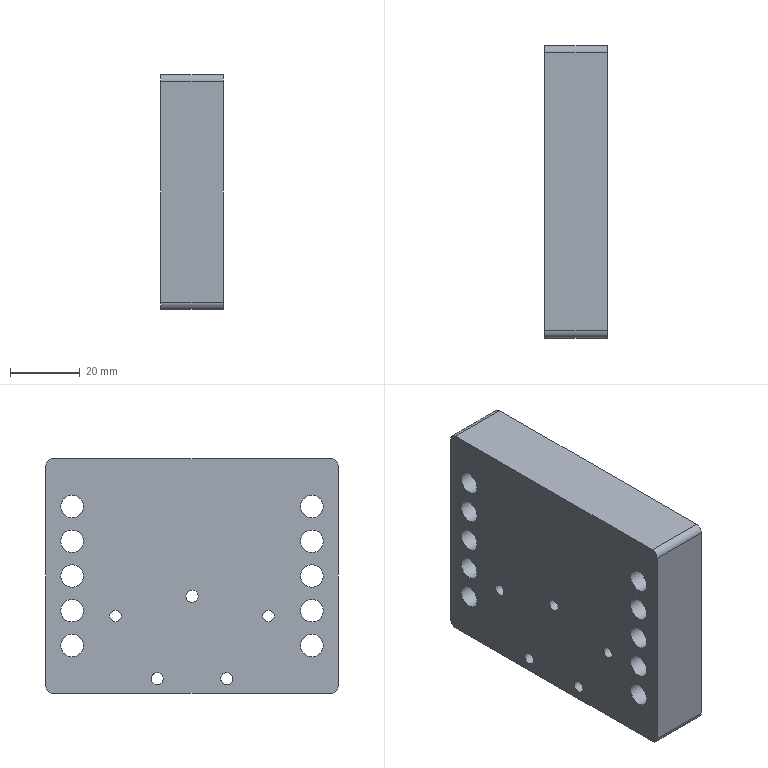CAM job | NX | 3+2 milling, drilling | part box 18 x 84 x 67.5 mm | stock box 20 x 89 x 72.5 mm
Tools:
number,name,description,diameter,corner_radius,flute_length,length,flutes
4,D4,平底铣刀-粗,4.0,0.0,25.0,75.0,2
9,D10,平底铣刀-粗,10.0,0.0,35.0,75.0,2
10,D10-J,平底铣刀-精,10.0,0.0,35.0,75.0,2
1,D80R0.8飞刀,圆鼻刀-粗,80.0,0.8,50.0,75.0,2
1,D80R0.8飞刀-J,圆鼻刀-精,80.0,0.8,50.0,75.0,2
2,D6倒角刀,倒角刀,6.0,0.0,3.0,25.0,2
21,M4X0.7,丝锥,3.3,0.0,35.0,50.0,2
17,ZT3.5,钻头,3.5,0.0,35.0,50.0,2
18,ZT6.5,钻头,6.5,0.0,35.0,50.0,2
13,DRILL3.3,Twist Drill 3.3 mm,3.3,0.0,35.0,35.008,2
Operations:
program,operation,operation_type,tool,method,geometry_group,spindle_rpm,surface_speed,feed_per_tooth,feed_cut,feed_plunge,cut_length_mm,path_length_mm,cut_time_min,machine_time_min
B,底壁铣飞面一刀开粗_COPY,VolumeBased25DMillingOperation,D80R0.8飞刀,分层开粗-切深K-步距G,W-B,2800.0,703.696,0.5357,3000.0,100.0,768.937,1368.017,0.2563,0.3162
B,底壁铣飞面一刀精光_COPY,VolumeBased25DMillingOperation,D80R0.8飞刀-J,侧刃精光-切深K-步距G,W-B,4000.0,1005.28,0.125,1000.0,100.0,192.038,228.038,0.192,0.1956
B,铣沉头_1,CylinderMilling,D4,METHOD,W-B,8000.0,100.531,0.075,1200.0,100.0,578.816,761.64,0.4823,0.5006
B,铣孔_1,CylinderMilling,D4,METHOD,W-B,8000.0,100.531,0.0375,600.0,100.0,55.559,257.282,0.0926,0.1128
B,钻倒角_3,Operation,D6倒角刀,METHOD,W-B,8000.0,150.796,0.0625,1000.0,0.0,10.4,107.902,0.0104,0.0202
B,铣倒角_2,PlanarMilling,D6倒角刀,METHOD,W-B,8000.0,150.796,0.0375,600.0,100.0,35.349,209.851,0.0589,0.0764
B,铣倒角_3,PlanarMilling,D6倒角刀,METHOD,W-B,8000.0,150.796,0.075,1200.0,100.0,201.908,772.78,0.1683,0.2253
B,C0.3封闭铣廓倒角6X45L_COPY,PlanarMilling,D6倒角刀,爬面_倒角-切深0-步距G,W-B,7000.0,131.0,0.1071,1500.0,100.0,317.198,353.198,0.2115,0.2151
A,顶面,FaceMilling,D80R0.8飞刀,侧刃精光-切深K-步距G,W-A,4000.0,1005.31,0.125,1000.0,100.0,178.0,214.0,0.178,0.1816
A,外形粗_2,VolumeBased25DMillingOperation,D10,METHOD,W-A,8000.0,251.327,0.3125,5000.0,80.0,8291.787,8348.387,1.658,1.664
A,打点-深0.8,Operation,D6倒角刀,NONE,W-A,8000.0,150.796,0.0312,500.0,90.0,27.0,308.899,0.054,0.0822
A,通孔-M4螺纹底孔,Operation,DRILL3.3,NONE,W-A,3000.0,31.102,0.05,300.0,90.0,49.983,184.977,0.1666,0.1801
A,通孔-3-4,Operation,ZT3.5,NONE,W-A,3000.0,32.987,0.02,120.0,90.0,66.0,219.768,0.55,0.5654
A,通孔-6-8,Operation,ZT6.5,NONE,W-A,2500.0,51.051,0.03,150.0,90.0,229.528,657.462,1.53,1.573
A,仅选体,SurfaceContour,D6倒角刀,METHOD,W-A,8000.0,150.796,0.1875,3000.0,100.0,315.596,350.797,0.1052,0.1087
A,钻倒角_1,Operation,D6倒角刀,METHOD,W-A,8000.0,150.796,0.0312,500.0,0.0,10.4,107.902,0.0208,0.0306
A,钻倒角_2,Operation,D6倒角刀,METHOD,W-A,8000.0,150.796,0.0312,500.0,0.0,15.15,122.421,0.0303,0.041
A,铣倒角_1,PlanarMilling,D6倒角刀,METHOD,W-A,8000.0,150.796,0.05,800.0,100.0,230.535,790.057,0.2882,0.3441
A,通孔-攻牙M4,Operation,M4X0.7,METHOD,W-A,600.0,6.22,0.0006,0.7,90.0,44.0,173.011,62.857,62.87
A,外形半精_2,VolumeBased25DMillingOperation,D10-J,METHOD,W-A,8000.0,251.327,0.0625,1000.0,100.0,335.961,411.161,0.336,0.3435